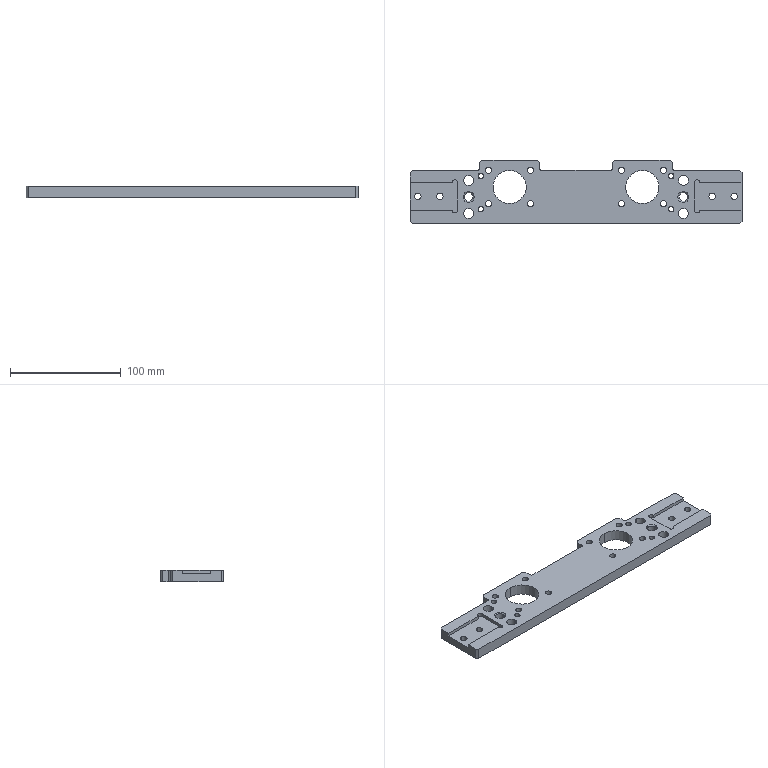Part | STEP file | J454-EBZ05-22-00-Part-1 | 1 solid | 128 faces | box 300 x 57 x 10 mm | volume 123602 mm3 | cylinder 82 | plane 42 | cone 4 | commonest cylinder face diameters 5.5 x16 9.5 x16 5 x14 4.5 x8 6 x8 9 x8